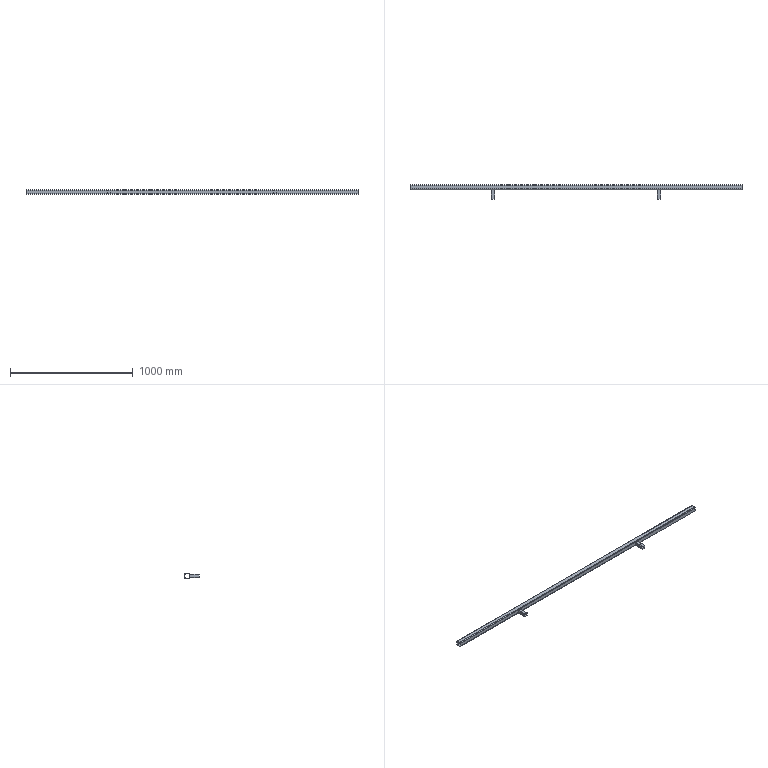Part | SolidWorks | features WeldMemberFeat 2, 3DProfileFeature 1, WeldCornerFeat 1, WeldmentFeature 1 | 3 solids | 54 faces | box 2700 x 120 x 40 mm | volume 1184354 mm3 | plane 30 | cylinder 24 | commonest cylinder face diameters 6 x12 12 x12